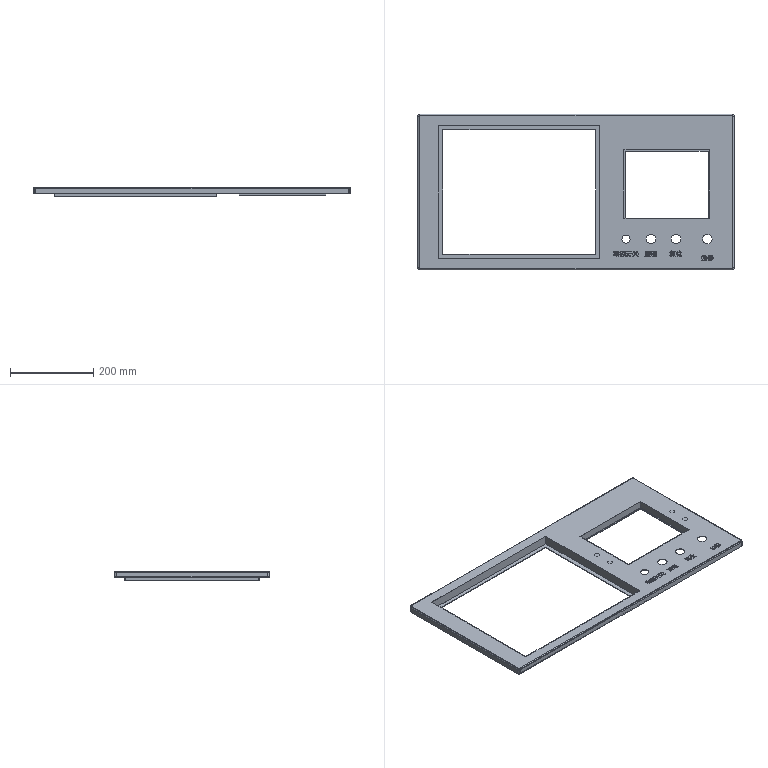Part | SolidWorks | features ICE 12, HoleWzd 3, Fillet 2, Extrusion 1, Shell 1 | 9 solids | 651 faces | box 758 x 373 x 23.5 mm | volume 379988 mm3 | plane 440 | spline 135 | cylinder 64 | cone 8 | torus 4 | commonest cylinder face diameters 3.3 x24 5 x16 12 x8 22.5 x6 6 x4 10 x4